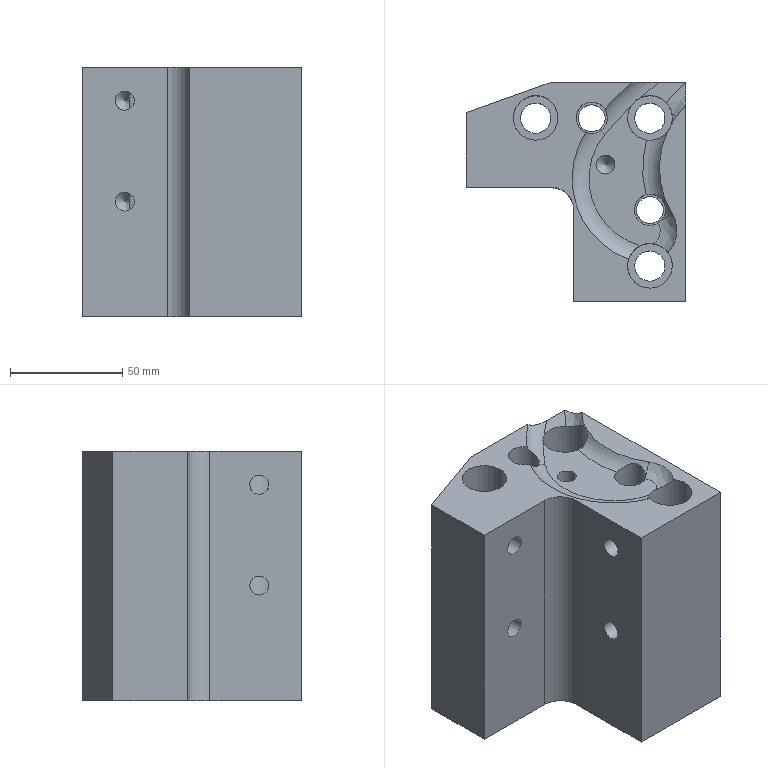Part | NX | features solid 2 | 1 solid | 41 faces | box 98 x 98 x 111.5 mm | volume 634006 mm3 | cylinder 16 | plane 16 | torus 4 | cone 3 | spline 2 | commonest cylinder face diameters 8.5 x5 20 x4 13.5 x3 12.001 x2 14 x2